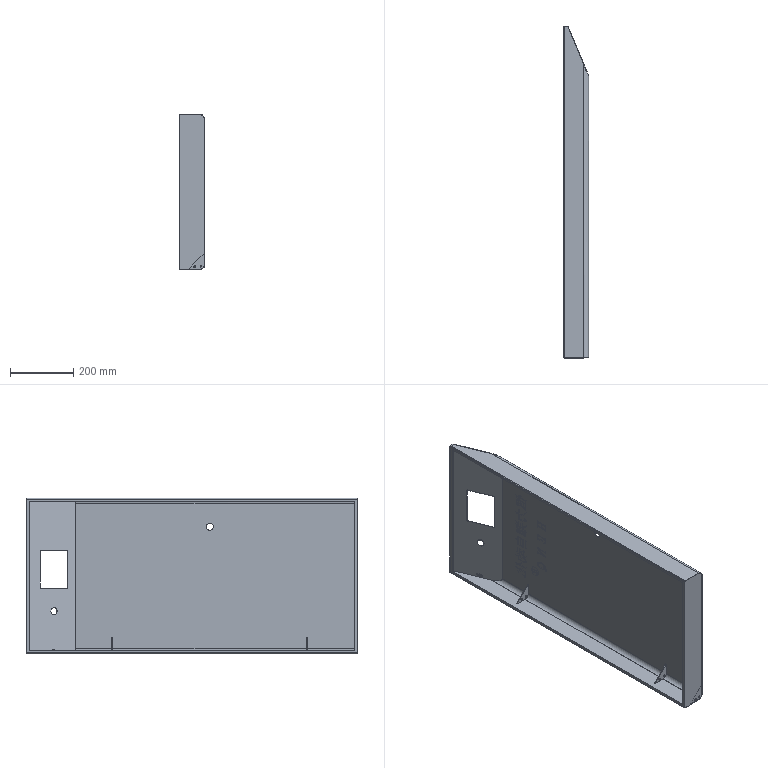Part | SolidWorks | features ICE 11, Fillet 2, Cut 1, HoleWzd 1, Shell 1 | 2 solids | 499 faces | box 80 x 1053 x 493 mm | volume 1093617 mm3 | plane 332 | spline 134 | cylinder 33 | commonest cylinder face diameters 7 x10 6.2 x6 22.5 x4 30 x3 3 x2 6 x2